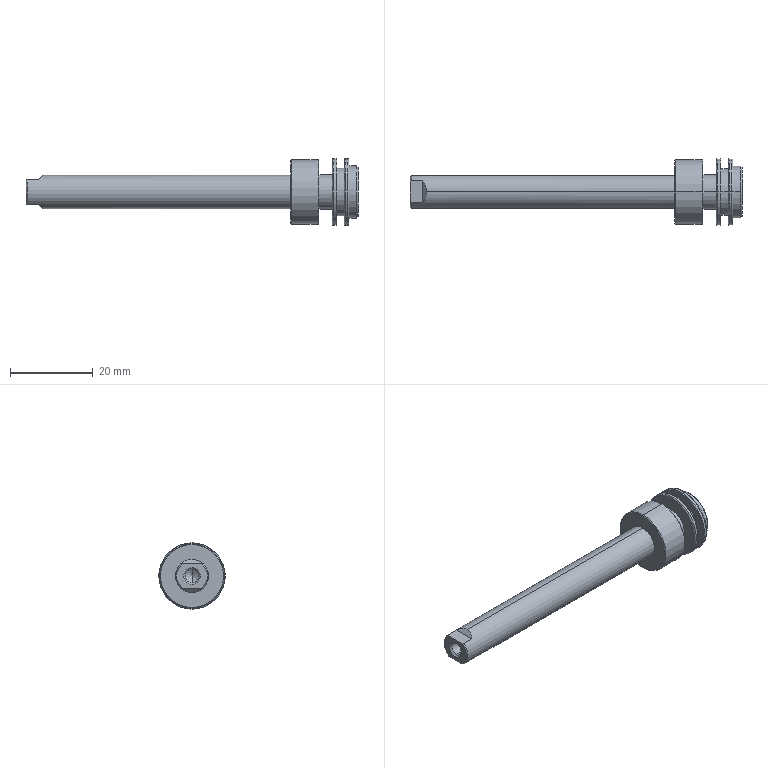Part | STEP file | ACQ16x50S-02-cc | 1 solid | 48 faces | box 80 x 16 x 16 mm | volume 5471 mm3 | cylinder 16 | cone 12 | plane 12 | spline 8 | commonest cylinder face diameters 16 x4 3.242 x2 8 x2 8.4 x2 11.4 x2 12.6 x2